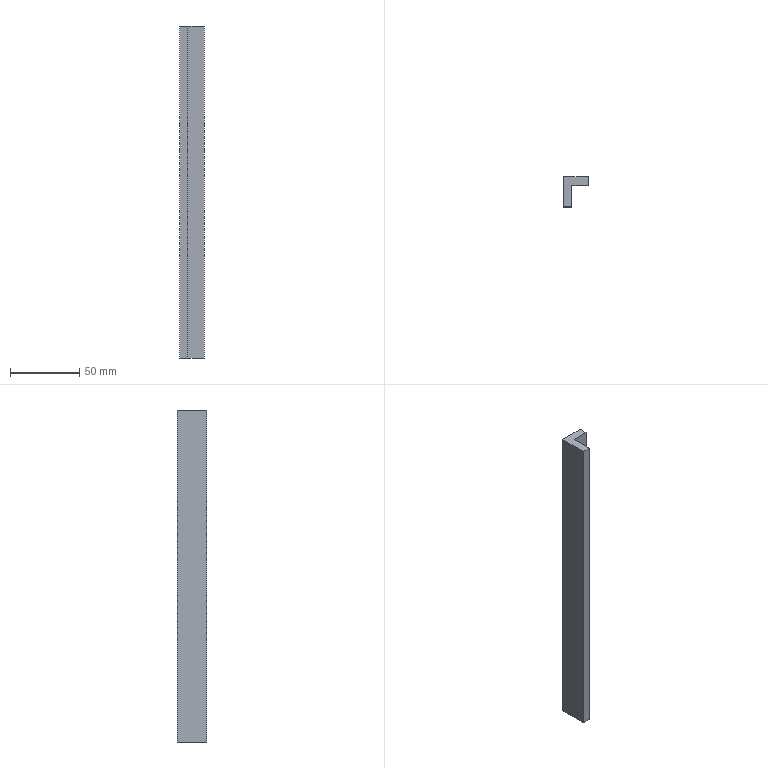Part | NX | 1 solid | 8 faces | box 18 x 21.457 x 240 mm | volume 48179 mm3 | plane 8
STEP:
#1=CARTESIAN_POINT('',(32.874,-598.957,2497.086));
#2=VERTEX_POINT('',#1);
#3=CARTESIAN_POINT('',(38.874,-598.957,2497.086));
#4=VERTEX_POINT('',#3);
#5=CARTESIAN_POINT('',(32.874,-598.957,2497.086));
#6=DIRECTION('',(1.,0.,0.));
#7=VECTOR('',#6,1.);
#8=LINE('',#5,#7);
#9=EDGE_CURVE('',#2,#4,#8,.T.);
#10=ORIENTED_EDGE('',*,*,#9,.F.);
#11=CARTESIAN_POINT('',(32.874,-598.957,2257.086));
#12=VERTEX_POINT('',#11);
#13=CARTESIAN_POINT('',(32.874,-598.957,2257.086));
#14=DIRECTION('',(0.,0.,1.));
#15=VECTOR('',#14,1.);
#16=LINE('',#13,#15);
#17=EDGE_CURVE('',#12,#2,#16,.T.);
#18=ORIENTED_EDGE('',*,*,#17,.F.);
#19=CARTESIAN_POINT('',(38.874,-598.957,2257.086));
#20=VERTEX_POINT('',#19);
#21=CARTESIAN_POINT('',(32.874,-598.957,2257.086));
#22=DIRECTION('',(1.,0.,0.));
#23=VECTOR('',#22,1.);
#24=LINE('',#21,#23);
#25=EDGE_CURVE('',#12,#20,#24,.T.);
#26=ORIENTED_EDGE('',*,*,#25,.T.);
#27=CARTESIAN_POINT('',(38.874,-598.957,2257.086));
#28=DIRECTION('',(0.,0.,1.));
#29=VECTOR('',#28,1.);
#30=LINE('',#27,#29);
#31=EDGE_CURVE('',#20,#4,#30,.T.);
#32=ORIENTED_EDGE('',*,*,#31,.T.);
#33=EDGE_LOOP('',(#10,#18,#26,#32));
#34=FACE_OUTER_BOUND('',#33,.T.);
#35=CARTESIAN_POINT('',(32.874,-598.957,2257.086));
#36=DIRECTION('',(0.,-1.,0.));
#37=DIRECTION('',(0.,0.,-1.));
#38=AXIS2_PLACEMENT_3D('',#35,#36,#37);
#39=PLANE('',#38);
#40=ADVANCED_FACE('',(#34),#39,.T.);
#41=CARTESIAN_POINT('',(32.874,-577.499,2497.086));
#42=VERTEX_POINT('',#41);
#43=CARTESIAN_POINT('',(32.874,-598.957,2497.086));
#44=DIRECTION('',(0.,-1.,0.));
#45=VECTOR('',#44,1.);
#46=LINE('',#43,#45);
#47=EDGE_CURVE('',#42,#2,#46,.T.);
#48=ORIENTED_EDGE('',*,*,#47,.F.);
#49=CARTESIAN_POINT('',(32.874,-577.499,2257.086));
#50=VERTEX_POINT('',#49);
#51=CARTESIAN_POINT('',(32.874,-577.499,2257.086));
#52=DIRECTION('',(0.,0.,1.));
#53=VECTOR('',#52,1.);
#54=LINE('',#51,#53);
#55=EDGE_CURVE('',#50,#42,#54,.T.);
#56=ORIENTED_EDGE('',*,*,#55,.F.);
#57=CARTESIAN_POINT('',(32.874,-598.957,2257.086));
#58=DIRECTION('',(0.,-1.,0.));
#59=VECTOR('',#58,1.);
#60=LINE('',#57,#59);
#61=EDGE_CURVE('',#50,#12,#60,.T.);
#62=ORIENTED_EDGE('',*,*,#61,.T.);
#63=ORIENTED_EDGE('',*,*,#17,.T.);
#64=EDGE_LOOP('',(#48,#56,#62,#63));
#65=FACE_OUTER_BOUND('',#64,.T.);
#66=CARTESIAN_POINT('',(32.874,-598.957,2257.086));
#67=DIRECTION('',(-1.,0.,0.));
#68=DIRECTION('',(0.,0.,1.));
#69=AXIS2_PLACEMENT_3D('',#66,#67,#68);
#70=PLANE('',#69);
#71=ADVANCED_FACE('',(#65),#70,.T.);
#72=CARTESIAN_POINT('',(50.874,-577.499,2497.086));
#73=VERTEX_POINT('',#72);
#74=CARTESIAN_POINT('',(32.874,-577.499,2497.086));
#75=DIRECTION('',(-1.,0.,0.));
#76=VECTOR('',#75,1.);
#77=LINE('',#74,#76);
#78=EDGE_CURVE('',#73,#42,#77,.T.);
#79=ORIENTED_EDGE('',*,*,#78,.F.);
#80=CARTESIAN_POINT('',(50.874,-577.499,2257.086));
#81=VERTEX_POINT('',#80);
#82=CARTESIAN_POINT('',(50.874,-577.499,2257.086));
#83=DIRECTION('',(0.,0.,1.));
#84=VECTOR('',#83,1.);
#85=LINE('',#82,#84);
#86=EDGE_CURVE('',#81,#73,#85,.T.);
#87=ORIENTED_EDGE('',*,*,#86,.F.);
#88=CARTESIAN_POINT('',(32.874,-577.499,2257.086));
#89=DIRECTION('',(-1.,0.,0.));
#90=VECTOR('',#89,1.);
#91=LINE('',#88,#90);
#92=EDGE_CURVE('',#81,#50,#91,.T.);
#93=ORIENTED_EDGE('',*,*,#92,.T.);
#94=ORIENTED_EDGE('',*,*,#55,.T.);
#95=EDGE_LOOP('',(#79,#87,#93,#94));
#96=FACE_OUTER_BOUND('',#95,.T.);
#97=CARTESIAN_POINT('',(32.874,-577.499,2257.086));
#98=DIRECTION('',(0.,1.,0.));
#99=DIRECTION('',(-1.,0.,0.));
#100=AXIS2_PLACEMENT_3D('',#97,#98,#99);
#101=PLANE('',#100);
#102=ADVANCED_FACE('',(#96),#101,.T.);
#103=CARTESIAN_POINT('',(50.874,-583.499,2497.086));
#104=VERTEX_POINT('',#103);
#105=CARTESIAN_POINT('',(50.874,-577.499,2497.086));
#106=DIRECTION('',(0.,1.,0.));
#107=VECTOR('',#106,1.);
#108=LINE('',#105,#107);
#109=EDGE_CURVE('',#104,#73,#108,.T.);
#110=ORIENTED_EDGE('',*,*,#109,.F.);
#111=CARTESIAN_POINT('',(50.874,-583.499,2257.086));
#112=VERTEX_POINT('',#111);
#113=CARTESIAN_POINT('',(50.874,-583.499,2257.086));
#114=DIRECTION('',(0.,0.,1.));
#115=VECTOR('',#114,1.);
#116=LINE('',#113,#115);
#117=EDGE_CURVE('',#112,#104,#116,.T.);
#118=ORIENTED_EDGE('',*,*,#117,.F.);
#119=CARTESIAN_POINT('',(50.874,-577.499,2257.086));
#120=DIRECTION('',(0.,1.,0.));
#121=VECTOR('',#120,1.);
#122=LINE('',#119,#121);
#123=EDGE_CURVE('',#112,#81,#122,.T.);
#124=ORIENTED_EDGE('',*,*,#123,.T.);
#125=ORIENTED_EDGE('',*,*,#86,.T.);
#126=EDGE_LOOP('',(#110,#118,#124,#125));
#127=FACE_OUTER_BOUND('',#126,.T.);
#128=CARTESIAN_POINT('',(50.874,-577.499,2257.086));
#129=DIRECTION('',(1.,0.,0.));
#130=DIRECTION('',(0.,1.,0.));
#131=AXIS2_PLACEMENT_3D('',#128,#129,#130);
#132=PLANE('',#131);
#133=ADVANCED_FACE('',(#127),#132,.T.);
#134=CARTESIAN_POINT('',(38.874,-583.499,2497.086));
#135=VERTEX_POINT('',#134);
#136=CARTESIAN_POINT('',(50.874,-583.499,2497.086));
#137=DIRECTION('',(1.,0.,0.));
#138=VECTOR('',#137,1.);
#139=LINE('',#136,#138);
#140=EDGE_CURVE('',#135,#104,#139,.T.);
#141=ORIENTED_EDGE('',*,*,#140,.F.);
#142=CARTESIAN_POINT('',(38.874,-583.499,2257.086));
#143=VERTEX_POINT('',#142);
#144=CARTESIAN_POINT('',(38.874,-583.499,2257.086));
#145=DIRECTION('',(0.,0.,1.));
#146=VECTOR('',#145,1.);
#147=LINE('',#144,#146);
#148=EDGE_CURVE('',#143,#135,#147,.T.);
#149=ORIENTED_EDGE('',*,*,#148,.F.);
#150=CARTESIAN_POINT('',(50.874,-583.499,2257.086));
#151=DIRECTION('',(1.,0.,0.));
#152=VECTOR('',#151,1.);
#153=LINE('',#150,#152);
#154=EDGE_CURVE('',#143,#112,#153,.T.);
#155=ORIENTED_EDGE('',*,*,#154,.T.);
#156=ORIENTED_EDGE('',*,*,#117,.T.);
#157=EDGE_LOOP('',(#141,#149,#155,#156));
#158=FACE_OUTER_BOUND('',#157,.T.);
#159=CARTESIAN_POINT('',(50.874,-583.499,2257.086));
#160=DIRECTION('',(0.,-1.,0.));
#161=DIRECTION('',(0.,0.,-1.));
#162=AXIS2_PLACEMENT_3D('',#159,#160,#161);
#163=PLANE('',#162);
#164=ADVANCED_FACE('',(#158),#163,.T.);
#165=CARTESIAN_POINT('',(38.874,-583.499,2497.086));
#166=DIRECTION('',(0.,1.,0.));
#167=VECTOR('',#166,1.);
#168=LINE('',#165,#167);
#169=EDGE_CURVE('',#4,#135,#168,.T.);
#170=ORIENTED_EDGE('',*,*,#169,.F.);
#171=ORIENTED_EDGE('',*,*,#31,.F.);
#172=CARTESIAN_POINT('',(38.874,-583.499,2257.086));
#173=DIRECTION('',(0.,1.,0.));
#174=VECTOR('',#173,1.);
#175=LINE('',#172,#174);
#176=EDGE_CURVE('',#20,#143,#175,.T.);
#177=ORIENTED_EDGE('',*,*,#176,.T.);
#178=ORIENTED_EDGE('',*,*,#148,.T.);
#179=EDGE_LOOP('',(#170,#171,#177,#178));
#180=FACE_OUTER_BOUND('',#179,.T.);
#181=CARTESIAN_POINT('',(38.874,-583.499,2257.086));
#182=DIRECTION('',(1.,0.,0.));
#183=DIRECTION('',(0.,1.,0.));
#184=AXIS2_PLACEMENT_3D('',#181,#182,#183);
#185=PLANE('',#184);
#186=ADVANCED_FACE('',(#180),#185,.T.);
#187=ORIENTED_EDGE('',*,*,#25,.F.);
#188=ORIENTED_EDGE('',*,*,#61,.F.);
#189=ORIENTED_EDGE('',*,*,#92,.F.);
#190=ORIENTED_EDGE('',*,*,#123,.F.);
#191=ORIENTED_EDGE('',*,*,#154,.F.);
#192=ORIENTED_EDGE('',*,*,#176,.F.);
#193=EDGE_LOOP('',(#187,#188,#189,#190,#191,#192));
#194=FACE_OUTER_BOUND('',#193,.T.);
#195=CARTESIAN_POINT('',(32.874,-598.957,2257.086));
#196=DIRECTION('',(0.,0.,1.));
#197=DIRECTION('',(1.,0.,0.));
#198=AXIS2_PLACEMENT_3D('',#195,#196,#197);
#199=PLANE('',#198);
#200=ADVANCED_FACE('',(#194),#199,.F.);
#201=ORIENTED_EDGE('',*,*,#9,.T.);
#202=ORIENTED_EDGE('',*,*,#169,.T.);
#203=ORIENTED_EDGE('',*,*,#140,.T.);
#204=ORIENTED_EDGE('',*,*,#109,.T.);
#205=ORIENTED_EDGE('',*,*,#78,.T.);
#206=ORIENTED_EDGE('',*,*,#47,.T.);
#207=EDGE_LOOP('',(#201,#202,#203,#204,#205,#206));
#208=FACE_OUTER_BOUND('',#207,.T.);
#209=CARTESIAN_POINT('',(32.874,-598.957,2497.086));
#210=DIRECTION('',(0.,0.,1.));
#211=DIRECTION('',(1.,0.,0.));
#212=AXIS2_PLACEMENT_3D('',#209,#210,#211);
#213=PLANE('',#212);
#214=ADVANCED_FACE('',(#208),#213,.T.);
#215=CLOSED_SHELL('',(#40,#71,#102,#133,#164,#186,#200,#214));
#216=MANIFOLD_SOLID_BREP('',#215);
#217=(LENGTH_UNIT()NAMED_UNIT(*)SI_UNIT(.MILLI.,.METRE.));
#218=UNCERTAINTY_MEASURE_WITH_UNIT(LENGTH_MEASURE(0.00002),#217,'','');
#219=(NAMED_UNIT(*)PLANE_ANGLE_UNIT()SI_UNIT($,.RADIAN.));
#220=PLANE_ANGLE_MEASURE_WITH_UNIT(PLANE_ANGLE_MEASURE(0.01745),#219);
#221=DIMENSIONAL_EXPONENTS(0.,0.,0.,0.,0.,0.,0.);
#222=(CONVERSION_BASED_UNIT('DEGREE',#220)NAMED_UNIT(#221)PLANE_ANGLE_UNIT());
#223=(NAMED_UNIT(*)SI_UNIT($,.STERADIAN.)SOLID_ANGLE_UNIT());
#224=(GEOMETRIC_REPRESENTATION_CONTEXT(3)GLOBAL_UNCERTAINTY_ASSIGNED_CONTEXT((#218))GLOBAL_UNIT_ASSIGNED_CONTEXT((#217,#222,#223))REPRESENTATION_CONTEXT('',''));
#225=ADVANCED_BREP_SHAPE_REPRESENTATION('',(#216),#224);